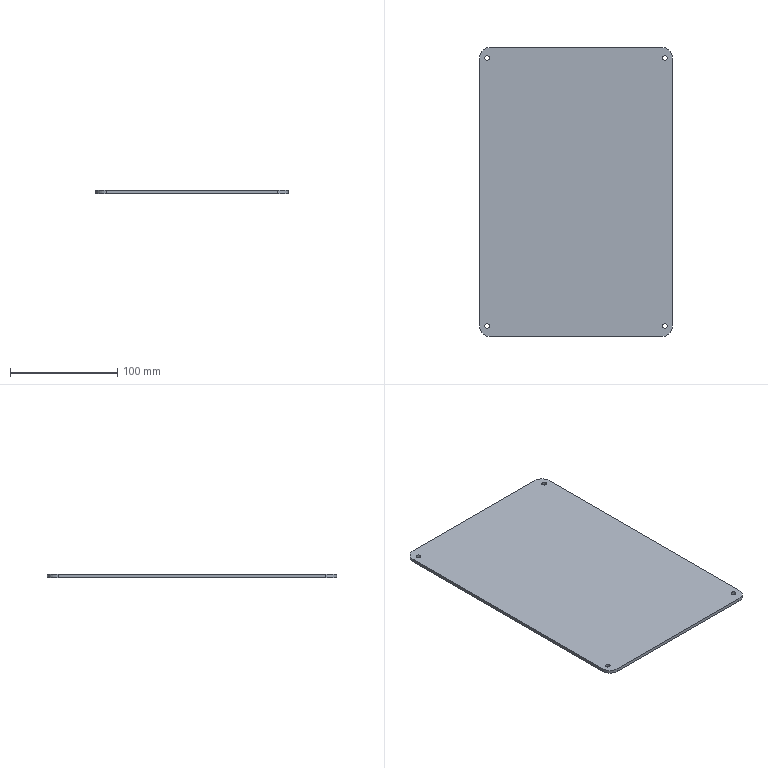Part | STEP file | Gear side cover plate SGN-2-31-01 | 1 solid | 18 faces | box 180 x 270 x 3 mm | volume 145368 mm3 | cylinder 12 | plane 6 | commonest cylinder face diameters 4.3 x8 20 x4